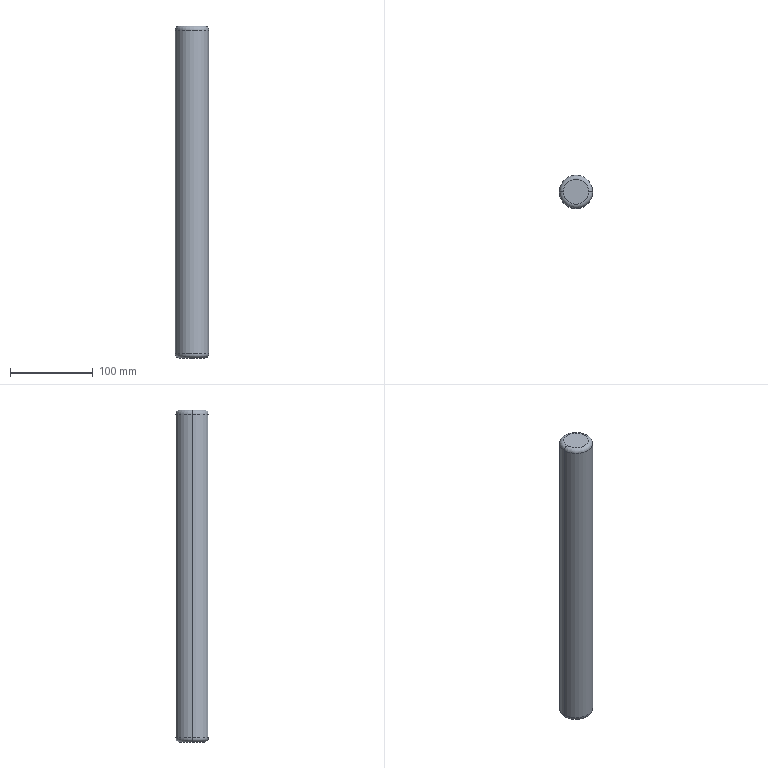Part | SolidWorks | features Extrusion 1, Fillet 1 | 1 solid | 8 faces | box 40 x 40 x 400 mm | volume 501382 mm3 | torus 4 | cylinder 2 | plane 2 | commonest cylinder face diameters 40 x2
STEP:
#1=CARTESIAN_POINT('',(-310.,235.,15.));
#2=VERTEX_POINT('',#1);
#3=CARTESIAN_POINT('',(-270.,235.,15.));
#4=VERTEX_POINT('',#3);
#5=CARTESIAN_POINT('',(-290.,235.,15.));
#6=DIRECTION('',(0.,0.,-1.));
#7=DIRECTION('',(1.,0.,0.));
#8=AXIS2_PLACEMENT_3D('',#5,#6,#7);
#9=CIRCLE('',#8,20.);
#10=EDGE_CURVE('',#2,#4,#9,.T.);
#11=ORIENTED_EDGE('',*,*,#10,.F.);
#12=CARTESIAN_POINT('',(-305.,235.,20.));
#13=VERTEX_POINT('',#12);
#14=CARTESIAN_POINT('',(-305.,235.,15.));
#15=DIRECTION('',(0.,1.,0.));
#16=DIRECTION('',(-1.,0.,0.));
#17=AXIS2_PLACEMENT_3D('',#14,#15,#16);
#18=CIRCLE('',#17,5.);
#19=EDGE_CURVE('',#2,#13,#18,.T.);
#20=ORIENTED_EDGE('',*,*,#19,.T.);
#21=CARTESIAN_POINT('',(-275.,235.,20.));
#22=VERTEX_POINT('',#21);
#23=CARTESIAN_POINT('',(-290.,235.,20.));
#24=DIRECTION('',(0.,0.,1.));
#25=DIRECTION('',(1.,0.,0.));
#26=AXIS2_PLACEMENT_3D('',#23,#24,#25);
#27=CIRCLE('',#26,15.);
#28=EDGE_CURVE('',#22,#13,#27,.T.);
#29=ORIENTED_EDGE('',*,*,#28,.F.);
#30=CARTESIAN_POINT('',(-275.,235.,15.));
#31=DIRECTION('',(0.,-1.,0.));
#32=DIRECTION('',(0.,0.,-1.));
#33=AXIS2_PLACEMENT_3D('',#30,#31,#32);
#34=CIRCLE('',#33,5.);
#35=EDGE_CURVE('',#4,#22,#34,.T.);
#36=ORIENTED_EDGE('',*,*,#35,.F.);
#37=EDGE_LOOP('',(#11,#20,#29,#36));
#38=FACE_OUTER_BOUND('',#37,.T.);
#39=CARTESIAN_POINT('',(-290.,235.,15.));
#40=DIRECTION('',(0.,0.,1.));
#41=DIRECTION('',(1.,0.,0.));
#42=AXIS2_PLACEMENT_3D('',#39,#40,#41);
#43=TOROIDAL_SURFACE('',#42,15.,5.);
#44=ADVANCED_FACE('',(#38),#43,.T.);
#45=CARTESIAN_POINT('',(-305.,235.,-380.));
#46=VERTEX_POINT('',#45);
#47=CARTESIAN_POINT('',(-275.,235.,-380.));
#48=VERTEX_POINT('',#47);
#49=CARTESIAN_POINT('',(-290.,235.,-380.));
#50=DIRECTION('',(0.,0.,-1.));
#51=DIRECTION('',(1.,0.,0.));
#52=AXIS2_PLACEMENT_3D('',#49,#50,#51);
#53=CIRCLE('',#52,15.);
#54=EDGE_CURVE('',#46,#48,#53,.T.);
#55=ORIENTED_EDGE('',*,*,#54,.F.);
#56=CARTESIAN_POINT('',(-310.,235.,-375.));
#57=VERTEX_POINT('',#56);
#58=CARTESIAN_POINT('',(-305.,235.,-375.));
#59=DIRECTION('',(0.,1.,0.));
#60=DIRECTION('',(-1.,0.,0.));
#61=AXIS2_PLACEMENT_3D('',#58,#59,#60);
#62=CIRCLE('',#61,5.);
#63=EDGE_CURVE('',#46,#57,#62,.T.);
#64=ORIENTED_EDGE('',*,*,#63,.T.);
#65=CARTESIAN_POINT('',(-270.,235.,-375.));
#66=VERTEX_POINT('',#65);
#67=CARTESIAN_POINT('',(-290.,235.,-375.));
#68=DIRECTION('',(0.,0.,1.));
#69=DIRECTION('',(1.,0.,0.));
#70=AXIS2_PLACEMENT_3D('',#67,#68,#69);
#71=CIRCLE('',#70,20.);
#72=EDGE_CURVE('',#66,#57,#71,.T.);
#73=ORIENTED_EDGE('',*,*,#72,.F.);
#74=CARTESIAN_POINT('',(-275.,235.,-375.));
#75=DIRECTION('',(0.,-1.,0.));
#76=DIRECTION('',(0.,0.,-1.));
#77=AXIS2_PLACEMENT_3D('',#74,#75,#76);
#78=CIRCLE('',#77,5.);
#79=EDGE_CURVE('',#48,#66,#78,.T.);
#80=ORIENTED_EDGE('',*,*,#79,.F.);
#81=EDGE_LOOP('',(#55,#64,#73,#80));
#82=FACE_OUTER_BOUND('',#81,.T.);
#83=CARTESIAN_POINT('',(-290.,235.,-375.));
#84=DIRECTION('',(0.,0.,1.));
#85=DIRECTION('',(1.,0.,0.));
#86=AXIS2_PLACEMENT_3D('',#83,#84,#85);
#87=TOROIDAL_SURFACE('',#86,15.,5.);
#88=ADVANCED_FACE('',(#82),#87,.T.);
#89=ORIENTED_EDGE('',*,*,#72,.T.);
#90=CARTESIAN_POINT('',(-310.,235.,-380.));
#91=DIRECTION('',(0.,0.,1.));
#92=VECTOR('',#91,1000.);
#93=LINE('',#90,#92);
#94=EDGE_CURVE('',#57,#2,#93,.T.);
#95=ORIENTED_EDGE('',*,*,#94,.T.);
#96=ORIENTED_EDGE('',*,*,#10,.T.);
#97=CARTESIAN_POINT('',(-270.,235.,-380.));
#98=DIRECTION('',(0.,0.,1.));
#99=VECTOR('',#98,1000.);
#100=LINE('',#97,#99);
#101=EDGE_CURVE('',#66,#4,#100,.T.);
#102=ORIENTED_EDGE('',*,*,#101,.F.);
#103=EDGE_LOOP('',(#89,#95,#96,#102));
#104=FACE_OUTER_BOUND('',#103,.T.);
#105=CARTESIAN_POINT('',(-290.,235.,-380.));
#106=DIRECTION('',(0.,0.,1.));
#107=DIRECTION('',(1.,0.,0.));
#108=AXIS2_PLACEMENT_3D('',#105,#106,#107);
#109=CYLINDRICAL_SURFACE('',#108,20.);
#110=ADVANCED_FACE('',(#104),#109,.T.);
#111=ORIENTED_EDGE('',*,*,#94,.F.);
#112=CARTESIAN_POINT('',(-290.,235.,-375.));
#113=DIRECTION('',(0.,0.,1.));
#114=DIRECTION('',(1.,0.,0.));
#115=AXIS2_PLACEMENT_3D('',#112,#113,#114);
#116=CIRCLE('',#115,20.);
#117=EDGE_CURVE('',#57,#66,#116,.T.);
#118=ORIENTED_EDGE('',*,*,#117,.T.);
#119=ORIENTED_EDGE('',*,*,#101,.T.);
#120=CARTESIAN_POINT('',(-290.,235.,15.));
#121=DIRECTION('',(0.,0.,-1.));
#122=DIRECTION('',(1.,0.,0.));
#123=AXIS2_PLACEMENT_3D('',#120,#121,#122);
#124=CIRCLE('',#123,20.);
#125=EDGE_CURVE('',#4,#2,#124,.T.);
#126=ORIENTED_EDGE('',*,*,#125,.T.);
#127=EDGE_LOOP('',(#111,#118,#119,#126));
#128=FACE_OUTER_BOUND('',#127,.T.);
#129=CARTESIAN_POINT('',(-290.,235.,-380.));
#130=DIRECTION('',(0.,0.,1.));
#131=DIRECTION('',(1.,0.,0.));
#132=AXIS2_PLACEMENT_3D('',#129,#130,#131);
#133=CYLINDRICAL_SURFACE('',#132,20.);
#134=ADVANCED_FACE('',(#128),#133,.T.);
#135=CARTESIAN_POINT('',(-290.,235.,-380.));
#136=DIRECTION('',(0.,0.,-1.));
#137=DIRECTION('',(1.,0.,0.));
#138=AXIS2_PLACEMENT_3D('',#135,#136,#137);
#139=CIRCLE('',#138,15.);
#140=EDGE_CURVE('',#48,#46,#139,.T.);
#141=ORIENTED_EDGE('',*,*,#140,.T.);
#142=ORIENTED_EDGE('',*,*,#54,.T.);
#143=EDGE_LOOP('',(#141,#142));
#144=FACE_OUTER_BOUND('',#143,.T.);
#145=CARTESIAN_POINT('',(-290.,235.,-380.));
#146=DIRECTION('',(0.,0.,1.));
#147=DIRECTION('',(1.,0.,0.));
#148=AXIS2_PLACEMENT_3D('',#145,#146,#147);
#149=PLANE('',#148);
#150=ADVANCED_FACE('',(#144),#149,.F.);
#151=ORIENTED_EDGE('',*,*,#28,.T.);
#152=CARTESIAN_POINT('',(-290.,235.,20.));
#153=DIRECTION('',(0.,0.,1.));
#154=DIRECTION('',(1.,0.,0.));
#155=AXIS2_PLACEMENT_3D('',#152,#153,#154);
#156=CIRCLE('',#155,15.);
#157=EDGE_CURVE('',#13,#22,#156,.T.);
#158=ORIENTED_EDGE('',*,*,#157,.T.);
#159=EDGE_LOOP('',(#151,#158));
#160=FACE_OUTER_BOUND('',#159,.T.);
#161=CARTESIAN_POINT('',(-290.,235.,20.));
#162=DIRECTION('',(0.,0.,1.));
#163=DIRECTION('',(1.,0.,0.));
#164=AXIS2_PLACEMENT_3D('',#161,#162,#163);
#165=PLANE('',#164);
#166=ADVANCED_FACE('',(#160),#165,.T.);
#167=ORIENTED_EDGE('',*,*,#63,.F.);
#168=ORIENTED_EDGE('',*,*,#140,.F.);
#169=ORIENTED_EDGE('',*,*,#79,.T.);
#170=ORIENTED_EDGE('',*,*,#117,.F.);
#171=EDGE_LOOP('',(#167,#168,#169,#170));
#172=FACE_OUTER_BOUND('',#171,.T.);
#173=CARTESIAN_POINT('',(-290.,235.,-375.));
#174=DIRECTION('',(0.,0.,1.));
#175=DIRECTION('',(1.,0.,0.));
#176=AXIS2_PLACEMENT_3D('',#173,#174,#175);
#177=TOROIDAL_SURFACE('',#176,15.,5.);
#178=ADVANCED_FACE('',(#172),#177,.T.);
#179=ORIENTED_EDGE('',*,*,#19,.F.);
#180=ORIENTED_EDGE('',*,*,#125,.F.);
#181=ORIENTED_EDGE('',*,*,#35,.T.);
#182=ORIENTED_EDGE('',*,*,#157,.F.);
#183=EDGE_LOOP('',(#179,#180,#181,#182));
#184=FACE_OUTER_BOUND('',#183,.T.);
#185=CARTESIAN_POINT('',(-290.,235.,15.));
#186=DIRECTION('',(0.,0.,1.));
#187=DIRECTION('',(1.,0.,0.));
#188=AXIS2_PLACEMENT_3D('',#185,#186,#187);
#189=TOROIDAL_SURFACE('',#188,15.,5.);
#190=ADVANCED_FACE('',(#184),#189,.T.);
#191=CLOSED_SHELL('',(#44,#88,#110,#134,#150,#166,#178,#190));
#192=MANIFOLD_SOLID_BREP('',#191);
#193=CARTESIAN_POINT('',(0.,0.,0.));
#194=DIRECTION('',(0.,0.,1.));
#195=DIRECTION('',(1.,0.,0.));
#196=AXIS2_PLACEMENT_3D('',#193,#194,#195);
#197=(LENGTH_UNIT()NAMED_UNIT(*)SI_UNIT(.MILLI.,.METRE.));
#198=UNCERTAINTY_MEASURE_WITH_UNIT(LENGTH_MEASURE(0.00001),#197,'','');
#199=(NAMED_UNIT(*)PLANE_ANGLE_UNIT()SI_UNIT($,.RADIAN.));
#200=(NAMED_UNIT(*)SI_UNIT($,.STERADIAN.)SOLID_ANGLE_UNIT());
#201=(GEOMETRIC_REPRESENTATION_CONTEXT(3)GLOBAL_UNCERTAINTY_ASSIGNED_CONTEXT((#198))GLOBAL_UNIT_ASSIGNED_CONTEXT((#197,#199,#200))REPRESENTATION_CONTEXT('',''));
#202=ADVANCED_BREP_SHAPE_REPRESENTATION('',(#192,#196),#201);